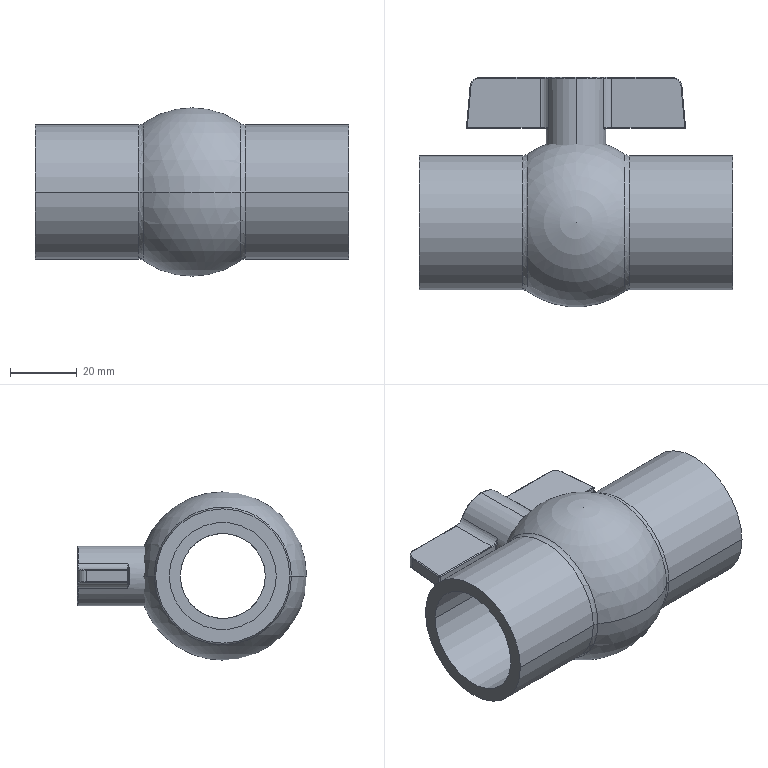Part | SolidWorks | features ICE 4, ConnectionPoint 2, Fillet 2, MoveFace 2, Revolution 2, MoveCopyBody 1, RoutePoint 1, Scale 1 | 3 solids | 95 faces | box 93.66 x 68.58 x 50.292 mm | volume 77419 mm3 | cylinder 37 | torus 25 | plane 15 | sphere 14 | spline 4 | commonest cylinder face diameters 0.508 x15 5.723 x6 25.4 x6 32.004 x4 40.132 x4 17.78 x2